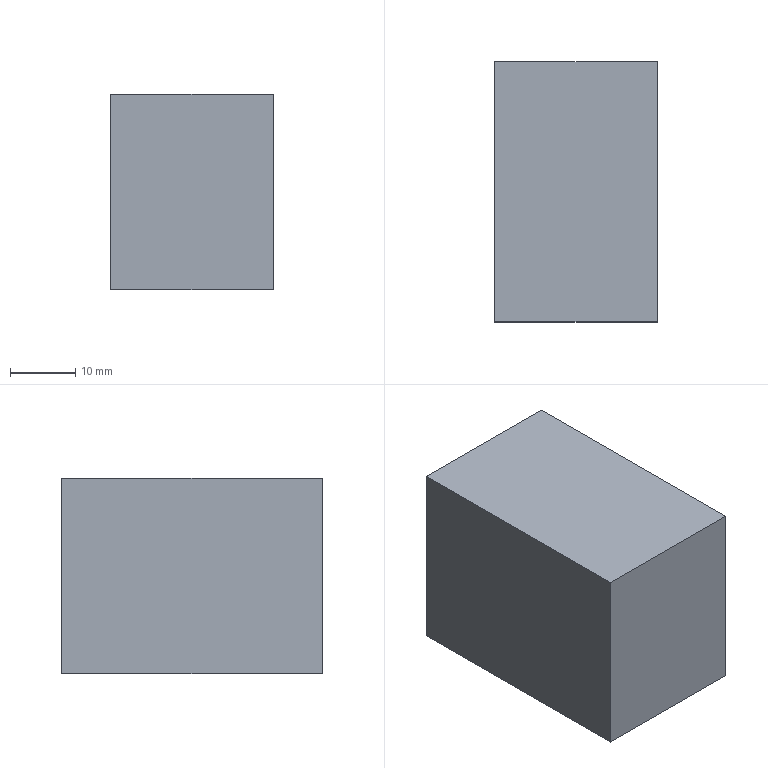Part | 1 solid | 6 faces | box 25 x 40 x 30 mm | volume 30000 mm3 | plane 6
STEP:
#1=CARTESIAN_POINT('',(0.,0.,0.));
#2=DIRECTION('',(0.,0.,1.));
#3=DIRECTION('',(1.,0.,0.));
#4=AXIS2_PLACEMENT_3D('',#1,#2,#3);
#5=CARTESIAN_POINT('',(-41.758,259.551,-256.55));
#6=VERTEX_POINT('',#5);
#7=CARTESIAN_POINT('',(-41.758,299.551,-256.55));
#8=VERTEX_POINT('',#7);
#9=CARTESIAN_POINT('',(-41.758,259.551,-256.55));
#10=DIRECTION('',(0.,1.,0.));
#11=VECTOR('',#10,1.);
#12=LINE('',#9,#11);
#13=CARTESIAN_POINT('',(-16.758,259.551,-256.55));
#14=DIRECTION('',(0.,0.,1.));
#15=DIRECTION('',(1.,0.,0.));
#16=AXIS2_PLACEMENT_3D('',#13,#14,#15);
#17=PLANE('',#16);
#18=CARTESIAN_POINT('',(-25.,0.));
#19=DIRECTION('',(0.,1.));
#20=VECTOR('',#19,1.);
#21=LINE('',#18,#20);
#22=(GEOMETRIC_REPRESENTATION_CONTEXT(2)PARAMETRIC_REPRESENTATION_CONTEXT()REPRESENTATION_CONTEXT('',''));
#23=DEFINITIONAL_REPRESENTATION('',(#21),#22);
#24=PCURVE('',#17,#23);
#25=CARTESIAN_POINT('',(-41.758,226.329,254.05));
#26=DIRECTION('',(-1.,0.,0.));
#27=DIRECTION('',(0.,0.,1.));
#28=AXIS2_PLACEMENT_3D('',#25,#26,#27);
#29=PLANE('',#28);
#30=CARTESIAN_POINT('',(-510.6,33.222));
#31=DIRECTION('',(0.,1.));
#32=VECTOR('',#31,1.);
#33=LINE('',#30,#32);
#34=(GEOMETRIC_REPRESENTATION_CONTEXT(2)PARAMETRIC_REPRESENTATION_CONTEXT()REPRESENTATION_CONTEXT('',''));
#35=DEFINITIONAL_REPRESENTATION('',(#33),#34);
#36=PCURVE('',#29,#35);
#37=SURFACE_CURVE('',#12,(#24,#36),.PCURVE_S1.);
#38=EDGE_CURVE('',#6,#8,#37,.T.);
#39=ORIENTED_EDGE('',*,*,#38,.F.);
#40=CARTESIAN_POINT('',(-16.758,259.551,-256.55));
#41=VERTEX_POINT('',#40);
#42=CARTESIAN_POINT('',(-16.758,259.551,-256.55));
#43=DIRECTION('',(-1.,0.,0.));
#44=VECTOR('',#43,1.);
#45=LINE('',#42,#44);
#46=CARTESIAN_POINT('',(0.,0.));
#47=DIRECTION('',(-1.,0.));
#48=VECTOR('',#47,1.);
#49=LINE('',#46,#48);
#50=(GEOMETRIC_REPRESENTATION_CONTEXT(2)PARAMETRIC_REPRESENTATION_CONTEXT()REPRESENTATION_CONTEXT('',''));
#51=DEFINITIONAL_REPRESENTATION('',(#49),#50);
#52=PCURVE('',#17,#51);
#53=CARTESIAN_POINT('',(-16.758,259.551,-286.55));
#54=DIRECTION('',(0.,-1.,0.));
#55=DIRECTION('',(0.,0.,-1.));
#56=AXIS2_PLACEMENT_3D('',#53,#54,#55);
#57=PLANE('',#56);
#58=CARTESIAN_POINT('',(-30.,0.));
#59=DIRECTION('',(0.,-1.));
#60=VECTOR('',#59,1.);
#61=LINE('',#58,#60);
#62=(GEOMETRIC_REPRESENTATION_CONTEXT(2)PARAMETRIC_REPRESENTATION_CONTEXT()REPRESENTATION_CONTEXT('',''));
#63=DEFINITIONAL_REPRESENTATION('',(#61),#62);
#64=PCURVE('',#57,#63);
#65=SURFACE_CURVE('',#45,(#52,#64),.PCURVE_S1.);
#66=EDGE_CURVE('',#41,#6,#65,.T.);
#67=ORIENTED_EDGE('',*,*,#66,.F.);
#68=CARTESIAN_POINT('',(-16.758,299.551,-256.55));
#69=VERTEX_POINT('',#68);
#70=CARTESIAN_POINT('',(-16.758,259.551,-256.55));
#71=DIRECTION('',(0.,1.,0.));
#72=VECTOR('',#71,1.);
#73=LINE('',#70,#72);
#74=CARTESIAN_POINT('',(0.,0.));
#75=DIRECTION('',(0.,1.));
#76=VECTOR('',#75,1.);
#77=LINE('',#74,#76);
#78=(GEOMETRIC_REPRESENTATION_CONTEXT(2)PARAMETRIC_REPRESENTATION_CONTEXT()REPRESENTATION_CONTEXT('',''));
#79=DEFINITIONAL_REPRESENTATION('',(#77),#78);
#80=PCURVE('',#17,#79);
#81=CARTESIAN_POINT('',(-16.758,226.329,254.05));
#82=DIRECTION('',(-1.,0.,0.));
#83=DIRECTION('',(0.,0.,1.));
#84=AXIS2_PLACEMENT_3D('',#81,#82,#83);
#85=PLANE('',#84);
#86=CARTESIAN_POINT('',(-510.6,33.222));
#87=DIRECTION('',(0.,1.));
#88=VECTOR('',#87,1.);
#89=LINE('',#86,#88);
#90=(GEOMETRIC_REPRESENTATION_CONTEXT(2)PARAMETRIC_REPRESENTATION_CONTEXT()REPRESENTATION_CONTEXT('',''));
#91=DEFINITIONAL_REPRESENTATION('',(#89),#90);
#92=PCURVE('',#85,#91);
#93=SURFACE_CURVE('',#73,(#80,#92),.PCURVE_S1.);
#94=EDGE_CURVE('',#41,#69,#93,.T.);
#95=ORIENTED_EDGE('',*,*,#94,.T.);
#96=CARTESIAN_POINT('',(-16.758,299.551,-256.55));
#97=DIRECTION('',(-1.,0.,0.));
#98=VECTOR('',#97,1.);
#99=LINE('',#96,#98);
#100=CARTESIAN_POINT('',(0.,40.));
#101=DIRECTION('',(-1.,0.));
#102=VECTOR('',#101,1.);
#103=LINE('',#100,#102);
#104=(GEOMETRIC_REPRESENTATION_CONTEXT(2)PARAMETRIC_REPRESENTATION_CONTEXT()REPRESENTATION_CONTEXT('',''));
#105=DEFINITIONAL_REPRESENTATION('',(#103),#104);
#106=PCURVE('',#17,#105);
#107=CARTESIAN_POINT('',(-16.758,299.551,-246.55));
#108=DIRECTION('',(0.,1.,0.));
#109=DIRECTION('',(0.,0.,1.));
#110=AXIS2_PLACEMENT_3D('',#107,#108,#109);
#111=PLANE('',#110);
#112=CARTESIAN_POINT('',(-10.,0.));
#113=DIRECTION('',(0.,-1.));
#114=VECTOR('',#113,1.);
#115=LINE('',#112,#114);
#116=(GEOMETRIC_REPRESENTATION_CONTEXT(2)PARAMETRIC_REPRESENTATION_CONTEXT()REPRESENTATION_CONTEXT('',''));
#117=DEFINITIONAL_REPRESENTATION('',(#115),#116);
#118=PCURVE('',#111,#117);
#119=SURFACE_CURVE('',#99,(#106,#118),.PCURVE_S1.);
#120=EDGE_CURVE('',#69,#8,#119,.T.);
#121=ORIENTED_EDGE('',*,*,#120,.T.);
#122=EDGE_LOOP('',(#39,#67,#95,#121));
#123=FACE_BOUND('',#122,.T.);
#124=ADVANCED_FACE('',(#123),#17,.T.);
#125=CARTESIAN_POINT('',(-41.758,299.551,-286.55));
#126=VERTEX_POINT('',#125);
#127=CARTESIAN_POINT('',(-41.758,299.551,-246.55));
#128=DIRECTION('',(0.,0.,-1.));
#129=VECTOR('',#128,1.);
#130=LINE('',#127,#129);
#131=CARTESIAN_POINT('',(0.,-25.));
#132=DIRECTION('',(-1.,0.));
#133=VECTOR('',#132,1.);
#134=LINE('',#131,#133);
#135=(GEOMETRIC_REPRESENTATION_CONTEXT(2)PARAMETRIC_REPRESENTATION_CONTEXT()REPRESENTATION_CONTEXT('',''));
#136=DEFINITIONAL_REPRESENTATION('',(#134),#135);
#137=PCURVE('',#111,#136);
#138=CARTESIAN_POINT('',(-500.6,73.222));
#139=DIRECTION('',(-1.,0.));
#140=VECTOR('',#139,1.);
#141=LINE('',#138,#140);
#142=(GEOMETRIC_REPRESENTATION_CONTEXT(2)PARAMETRIC_REPRESENTATION_CONTEXT()REPRESENTATION_CONTEXT('',''));
#143=DEFINITIONAL_REPRESENTATION('',(#141),#142);
#144=PCURVE('',#29,#143);
#145=SURFACE_CURVE('',#130,(#137,#144),.PCURVE_S1.);
#146=EDGE_CURVE('',#8,#126,#145,.T.);
#147=ORIENTED_EDGE('',*,*,#146,.F.);
#148=ORIENTED_EDGE('',*,*,#120,.F.);
#149=CARTESIAN_POINT('',(-16.758,299.551,-286.55));
#150=VERTEX_POINT('',#149);
#151=CARTESIAN_POINT('',(-16.758,299.551,-246.55));
#152=DIRECTION('',(0.,0.,-1.));
#153=VECTOR('',#152,1.);
#154=LINE('',#151,#153);
#155=CARTESIAN_POINT('',(0.,0.));
#156=DIRECTION('',(-1.,0.));
#157=VECTOR('',#156,1.);
#158=LINE('',#155,#157);
#159=(GEOMETRIC_REPRESENTATION_CONTEXT(2)PARAMETRIC_REPRESENTATION_CONTEXT()REPRESENTATION_CONTEXT('',''));
#160=DEFINITIONAL_REPRESENTATION('',(#158),#159);
#161=PCURVE('',#111,#160);
#162=CARTESIAN_POINT('',(-500.6,73.222));
#163=DIRECTION('',(-1.,0.));
#164=VECTOR('',#163,1.);
#165=LINE('',#162,#164);
#166=(GEOMETRIC_REPRESENTATION_CONTEXT(2)PARAMETRIC_REPRESENTATION_CONTEXT()REPRESENTATION_CONTEXT('',''));
#167=DEFINITIONAL_REPRESENTATION('',(#165),#166);
#168=PCURVE('',#85,#167);
#169=SURFACE_CURVE('',#154,(#161,#168),.PCURVE_S1.);
#170=EDGE_CURVE('',#69,#150,#169,.T.);
#171=ORIENTED_EDGE('',*,*,#170,.T.);
#172=CARTESIAN_POINT('',(-16.758,299.551,-286.55));
#173=DIRECTION('',(-1.,0.,0.));
#174=VECTOR('',#173,1.);
#175=LINE('',#172,#174);
#176=CARTESIAN_POINT('',(-40.,0.));
#177=DIRECTION('',(0.,-1.));
#178=VECTOR('',#177,1.);
#179=LINE('',#176,#178);
#180=(GEOMETRIC_REPRESENTATION_CONTEXT(2)PARAMETRIC_REPRESENTATION_CONTEXT()REPRESENTATION_CONTEXT('',''));
#181=DEFINITIONAL_REPRESENTATION('',(#179),#180);
#182=PCURVE('',#111,#181);
#183=CARTESIAN_POINT('',(-16.758,299.551,-286.55));
#184=DIRECTION('',(0.,0.,-1.));
#185=DIRECTION('',(-1.,0.,0.));
#186=AXIS2_PLACEMENT_3D('',#183,#184,#185);
#187=PLANE('',#186);
#188=CARTESIAN_POINT('',(0.,0.));
#189=DIRECTION('',(1.,0.));
#190=VECTOR('',#189,1.);
#191=LINE('',#188,#190);
#192=(GEOMETRIC_REPRESENTATION_CONTEXT(2)PARAMETRIC_REPRESENTATION_CONTEXT()REPRESENTATION_CONTEXT('',''));
#193=DEFINITIONAL_REPRESENTATION('',(#191),#192);
#194=PCURVE('',#187,#193);
#195=SURFACE_CURVE('',#175,(#182,#194),.PCURVE_S1.);
#196=EDGE_CURVE('',#150,#126,#195,.T.);
#197=ORIENTED_EDGE('',*,*,#196,.T.);
#198=EDGE_LOOP('',(#147,#148,#171,#197));
#199=FACE_BOUND('',#198,.T.);
#200=ADVANCED_FACE('',(#199),#111,.T.);
#201=CARTESIAN_POINT('',(-41.758,259.551,-286.55));
#202=VERTEX_POINT('',#201);
#203=CARTESIAN_POINT('',(-41.758,299.551,-286.55));
#204=DIRECTION('',(0.,-1.,0.));
#205=VECTOR('',#204,1.);
#206=LINE('',#203,#205);
#207=CARTESIAN_POINT('',(25.,0.));
#208=DIRECTION('',(0.,-1.));
#209=VECTOR('',#208,1.);
#210=LINE('',#207,#209);
#211=(GEOMETRIC_REPRESENTATION_CONTEXT(2)PARAMETRIC_REPRESENTATION_CONTEXT()REPRESENTATION_CONTEXT('',''));
#212=DEFINITIONAL_REPRESENTATION('',(#210),#211);
#213=PCURVE('',#187,#212);
#214=CARTESIAN_POINT('',(-540.6,73.222));
#215=DIRECTION('',(0.,-1.));
#216=VECTOR('',#215,1.);
#217=LINE('',#214,#216);
#218=(GEOMETRIC_REPRESENTATION_CONTEXT(2)PARAMETRIC_REPRESENTATION_CONTEXT()REPRESENTATION_CONTEXT('',''));
#219=DEFINITIONAL_REPRESENTATION('',(#217),#218);
#220=PCURVE('',#29,#219);
#221=SURFACE_CURVE('',#206,(#213,#220),.PCURVE_S1.);
#222=EDGE_CURVE('',#126,#202,#221,.T.);
#223=ORIENTED_EDGE('',*,*,#222,.F.);
#224=ORIENTED_EDGE('',*,*,#196,.F.);
#225=CARTESIAN_POINT('',(-16.758,259.551,-286.55));
#226=VERTEX_POINT('',#225);
#227=CARTESIAN_POINT('',(-16.758,299.551,-286.55));
#228=DIRECTION('',(0.,-1.,0.));
#229=VECTOR('',#228,1.);
#230=LINE('',#227,#229);
#231=CARTESIAN_POINT('',(0.,0.));
#232=DIRECTION('',(0.,-1.));
#233=VECTOR('',#232,1.);
#234=LINE('',#231,#233);
#235=(GEOMETRIC_REPRESENTATION_CONTEXT(2)PARAMETRIC_REPRESENTATION_CONTEXT()REPRESENTATION_CONTEXT('',''));
#236=DEFINITIONAL_REPRESENTATION('',(#234),#235);
#237=PCURVE('',#187,#236);
#238=CARTESIAN_POINT('',(-540.6,73.222));
#239=DIRECTION('',(0.,-1.));
#240=VECTOR('',#239,1.);
#241=LINE('',#238,#240);
#242=(GEOMETRIC_REPRESENTATION_CONTEXT(2)PARAMETRIC_REPRESENTATION_CONTEXT()REPRESENTATION_CONTEXT('',''));
#243=DEFINITIONAL_REPRESENTATION('',(#241),#242);
#244=PCURVE('',#85,#243);
#245=SURFACE_CURVE('',#230,(#237,#244),.PCURVE_S1.);
#246=EDGE_CURVE('',#150,#226,#245,.T.);
#247=ORIENTED_EDGE('',*,*,#246,.T.);
#248=CARTESIAN_POINT('',(-16.758,259.551,-286.55));
#249=DIRECTION('',(-1.,0.,0.));
#250=VECTOR('',#249,1.);
#251=LINE('',#248,#250);
#252=CARTESIAN_POINT('',(0.,-40.));
#253=DIRECTION('',(1.,0.));
#254=VECTOR('',#253,1.);
#255=LINE('',#252,#254);
#256=(GEOMETRIC_REPRESENTATION_CONTEXT(2)PARAMETRIC_REPRESENTATION_CONTEXT()REPRESENTATION_CONTEXT('',''));
#257=DEFINITIONAL_REPRESENTATION('',(#255),#256);
#258=PCURVE('',#187,#257);
#259=CARTESIAN_POINT('',(0.,0.));
#260=DIRECTION('',(0.,-1.));
#261=VECTOR('',#260,1.);
#262=LINE('',#259,#261);
#263=(GEOMETRIC_REPRESENTATION_CONTEXT(2)PARAMETRIC_REPRESENTATION_CONTEXT()REPRESENTATION_CONTEXT('',''));
#264=DEFINITIONAL_REPRESENTATION('',(#262),#263);
#265=PCURVE('',#57,#264);
#266=SURFACE_CURVE('',#251,(#258,#265),.PCURVE_S1.);
#267=EDGE_CURVE('',#226,#202,#266,.T.);
#268=ORIENTED_EDGE('',*,*,#267,.T.);
#269=EDGE_LOOP('',(#223,#224,#247,#268));
#270=FACE_BOUND('',#269,.T.);
#271=ADVANCED_FACE('',(#270),#187,.T.);
#272=CARTESIAN_POINT('',(-41.758,259.551,-286.55));
#273=DIRECTION('',(0.,0.,1.));
#274=VECTOR('',#273,1.);
#275=LINE('',#272,#274);
#276=CARTESIAN_POINT('',(0.,-25.));
#277=DIRECTION('',(-1.,0.));
#278=VECTOR('',#277,1.);
#279=LINE('',#276,#278);
#280=(GEOMETRIC_REPRESENTATION_CONTEXT(2)PARAMETRIC_REPRESENTATION_CONTEXT()REPRESENTATION_CONTEXT('',''));
#281=DEFINITIONAL_REPRESENTATION('',(#279),#280);
#282=PCURVE('',#57,#281);
#283=CARTESIAN_POINT('',(-540.6,33.222));
#284=DIRECTION('',(1.,0.));
#285=VECTOR('',#284,1.);
#286=LINE('',#283,#285);
#287=(GEOMETRIC_REPRESENTATION_CONTEXT(2)PARAMETRIC_REPRESENTATION_CONTEXT()REPRESENTATION_CONTEXT('',''));
#288=DEFINITIONAL_REPRESENTATION('',(#286),#287);
#289=PCURVE('',#29,#288);
#290=SURFACE_CURVE('',#275,(#282,#289),.PCURVE_S1.);
#291=EDGE_CURVE('',#202,#6,#290,.T.);
#292=ORIENTED_EDGE('',*,*,#291,.F.);
#293=ORIENTED_EDGE('',*,*,#267,.F.);
#294=CARTESIAN_POINT('',(-16.758,259.551,-286.55));
#295=DIRECTION('',(0.,0.,1.));
#296=VECTOR('',#295,1.);
#297=LINE('',#294,#296);
#298=CARTESIAN_POINT('',(0.,0.));
#299=DIRECTION('',(-1.,0.));
#300=VECTOR('',#299,1.);
#301=LINE('',#298,#300);
#302=(GEOMETRIC_REPRESENTATION_CONTEXT(2)PARAMETRIC_REPRESENTATION_CONTEXT()REPRESENTATION_CONTEXT('',''));
#303=DEFINITIONAL_REPRESENTATION('',(#301),#302);
#304=PCURVE('',#57,#303);
#305=CARTESIAN_POINT('',(-540.6,33.222));
#306=DIRECTION('',(1.,0.));
#307=VECTOR('',#306,1.);
#308=LINE('',#305,#307);
#309=(GEOMETRIC_REPRESENTATION_CONTEXT(2)PARAMETRIC_REPRESENTATION_CONTEXT()REPRESENTATION_CONTEXT('',''));
#310=DEFINITIONAL_REPRESENTATION('',(#308),#309);
#311=PCURVE('',#85,#310);
#312=SURFACE_CURVE('',#297,(#304,#311),.PCURVE_S1.);
#313=EDGE_CURVE('',#226,#41,#312,.T.);
#314=ORIENTED_EDGE('',*,*,#313,.T.);
#315=ORIENTED_EDGE('',*,*,#66,.T.);
#316=EDGE_LOOP('',(#292,#293,#314,#315));
#317=FACE_BOUND('',#316,.T.);
#318=ADVANCED_FACE('',(#317),#57,.T.);
#319=ORIENTED_EDGE('',*,*,#94,.F.);
#320=ORIENTED_EDGE('',*,*,#313,.F.);
#321=ORIENTED_EDGE('',*,*,#246,.F.);
#322=ORIENTED_EDGE('',*,*,#170,.F.);
#323=EDGE_LOOP('',(#319,#320,#321,#322));
#324=FACE_BOUND('',#323,.T.);
#325=ADVANCED_FACE('',(#324),#85,.F.);
#326=ORIENTED_EDGE('',*,*,#38,.T.);
#327=ORIENTED_EDGE('',*,*,#146,.T.);
#328=ORIENTED_EDGE('',*,*,#222,.T.);
#329=ORIENTED_EDGE('',*,*,#291,.T.);
#330=EDGE_LOOP('',(#326,#327,#328,#329));
#331=FACE_BOUND('',#330,.T.);
#332=ADVANCED_FACE('',(#331),#29,.T.);
#333=CLOSED_SHELL('',(#124,#200,#271,#318,#325,#332));
#334=MANIFOLD_SOLID_BREP('',#333);
#335=(LENGTH_UNIT()NAMED_UNIT(*)SI_UNIT(.MILLI.,.METRE.));
#336=UNCERTAINTY_MEASURE_WITH_UNIT(LENGTH_MEASURE(0.0000001),#335,'','');
#337=(NAMED_UNIT(*)PLANE_ANGLE_UNIT()SI_UNIT($,.RADIAN.));
#338=(NAMED_UNIT(*)SI_UNIT($,.STERADIAN.)SOLID_ANGLE_UNIT());
#339=(GEOMETRIC_REPRESENTATION_CONTEXT(3)GLOBAL_UNCERTAINTY_ASSIGNED_CONTEXT((#336))GLOBAL_UNIT_ASSIGNED_CONTEXT((#335,#337,#338))REPRESENTATION_CONTEXT('',''));
#340=ADVANCED_BREP_SHAPE_REPRESENTATION('',(#4,#334),#339);